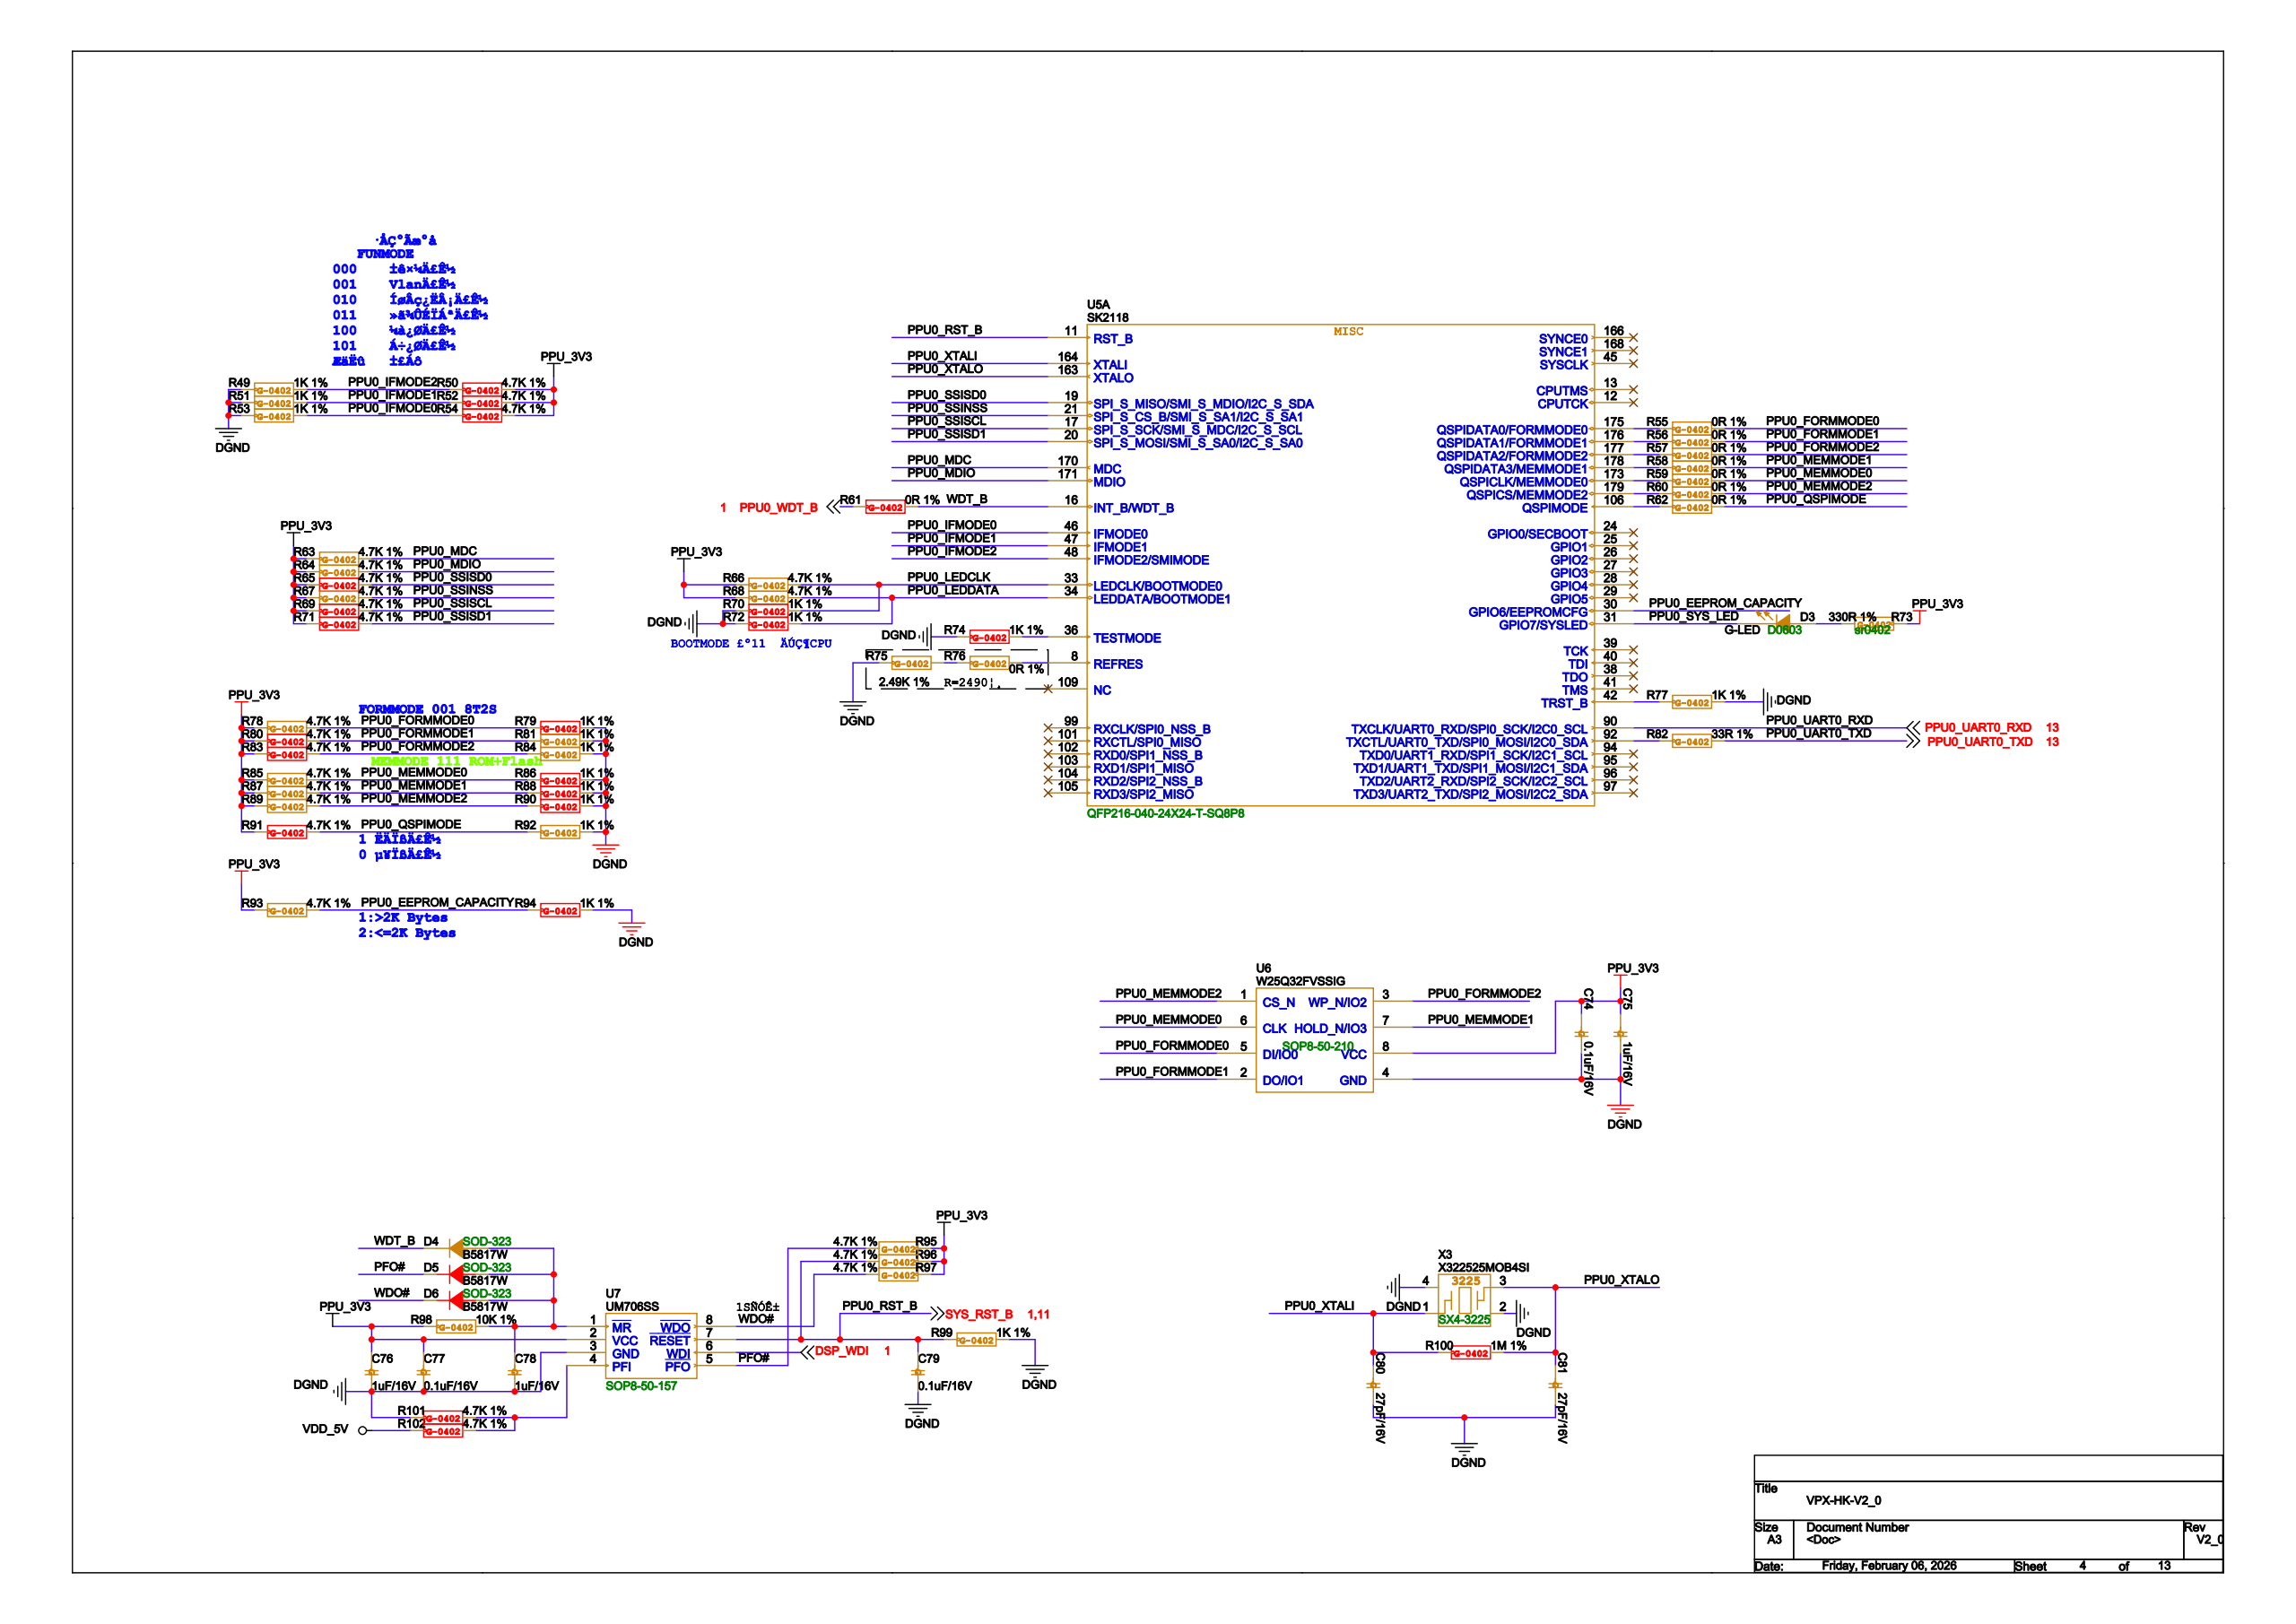Circuit board | Cadence Allegro | 598 parts | 541 nets | one sheet of the schematic
Parts on this sheet (reference | value | footprint):
C74 | 0.1uF/16V | SC0402
C75 | 1uF/16V | SC0402
C80 | 27pF/16V | SC0402
C81 | 27pF/16V | SC0402
D3 | G-LED | D0603
D4 | B5817W | SOD-323
D5 | B5817W | SOD-323
D6 | B5817W | SOD-323
R49 | 1K 1% | SR0402
R50 | 4.7K 1% | SR0402
R51 | 1K 1% | SR0402
R52 | 4.7K 1% | SR0402
R53 | 1K 1% | SR0402
R54 | 4.7K 1% | SR0402
R55 | 0R 1% | SR0402
R56 | 0R 1% | SR0402
R57 | 0R 1% | SR0402
R58 | 0R 1% | SR0402
R59 | 0R 1% | SR0402
R60 | 0R 1% | SR0402
R61 | 0R 1% | SR0402
R62 | 0R 1% | SR0402
R63 | 4.7K 1% | SR0402
R64 | 4.7K 1% | SR0402
R65 | 4.7K 1% | SR0402
R66 | 4.7K 1% | SR0402
R67 | 4.7K 1% | SR0402
R68 | 4.7K 1% | SR0402
R69 | 4.7K 1% | SR0402
R70 | 1K 1% | SR0402
R71 | 4.7K 1% | SR0402
R72 | 1K 1% | SR0402
R73 | 330R 1% | SR0402
R74 | 1K 1% | SR0402
R75 | 2.49K 1% | SR0402
R76 | 0R 1% | SR0402
R77 | 1K 1% | SR0402
R78 | 4.7K 1% | SR0402
R79 | 1K 1% | SR0402
R80 | 4.7K 1% | SR0402
R81 | 1K 1% | SR0402
R82 | 33R 1% | SR0402
R83 | 4.7K 1% | SR0402
R84 | 1K 1% | SR0402
R85 | 4.7K 1% | SR0402
R86 | 1K 1% | SR0402
R87 | 4.7K 1% | SR0402
R88 | 1K 1% | SR0402
R89 | 4.7K 1% | SR0402
R90 | 1K 1% | SR0402
R91 | 4.7K 1% | SR0402
R92 | 1K 1% | SR0402
R93 | 4.7K 1% | SR0402
R94 | 1K 1% | SR0402
R95 | 4.7K 1% | SR0402
R96 | 4.7K 1% | SR0402
R97 | 4.7K 1% | SR0402
R98 | 10K 1% | SR0402
R99 | 1K 1% | SR0402
R100 | 1M 1% | SR0402
R101 | 4.7K 1% | SR0402
R102 | 4.7K 1% | SR0402
U5 | SK2118 | QFP216-040-24X24-T-SQ8P8
U6 | W25Q32FVSSIG | SOP8-50-210
U7 | UM706SS | SOP8-50-157
X3 | X322525MOB4SI | SX4-3225
Nets of these parts (net: part-pin ...):
PPU_3V3: C74-1 C75-1 R50-2 R52-2 R54-2 R63-1 R64-1 R65-1 R66-1 R67-1 R68-1 R69-1 R71-1 R73-1 R78-1 R80-1 R83-1 R85-1 R87-1 R89-1 R91-1 R93-1 R95-1 R96-1 R97-1 R98-1 U6-8 U7-2
DGND: C74-2 C75-2 C80-2 C81-2 R49-1 R51-1 R53-1 R70-1 R72-1 R74-1 R75-1 R77-2 R79-2 R81-2 R84-2 R86-2 R88-2 R90-2 R92-2 R94-2 R99-2 R101-1 U6-4 U7-3 X3-2 X3-4 U5-7
VDD_5V: R102-1
N32613632: D4-2 D5-2 D6-2 R98-2 U7-1
PPU0_XTALI: C80-1 R100-1 X3-1 U5-164
PPU0_XTALO: C81-1 R100-2 X3-3 U5-163
DSP_WDI: U7-6
SYS_RST_B: R96-2 R99-1 U7-7 U5-11
WDT_B: D4-1 R61-2 U5-16
PFO#: D5-1 R95-2 U7-5
WDO#: D6-1 R97-2 U7-8
PPU0_UART0_TXD: R82-2
PPU0_UART0_RXD: U5-90
PPU0_WDT_B: R61-1
PPU0_EEPROM_CAPACITY: R93-2 R94-1 U5-30
PPU0_SYS_LED: D3-2 U5-31
PPU0_IFMODE0: R53-2 R54-1 U5-46
PPU0_IFMODE1: R51-2 R52-1 U5-47
PPU0_IFMODE2: R49-2 R50-1 U5-48
PPU0_LEDCLK: R66-2 R70-2 U5-33
PPU0_LEDDATA: R68-2 R72-2 U5-34
PPU0_MDC: R63-2 U5-170
PPU0_MDIO: R64-2 U5-171
N32613337: R59-1 U5-173
N32613339: R60-1 U5-179
N32613289: R55-1 U5-175
N32613291: R56-1 U5-176
N32613301: R57-1 U5-177
N32613319: R58-1 U5-178
N32613365: R62-1 U5-106
N32613186: R76-2 U5-8
PPU0_SSINSS: R67-2 U5-21
PPU0_SSISD0: R65-2 U5-19
PPU0_SSISD1: R71-2 U5-20
PPU0_SSISCL: R69-2 U5-17
N32613353: R74-2 U5-36
N32613188: R77-1 U5-42
N32613392: R82-1 U5-92
N32843620: R101-2 R102-2 U7-4
N32915429: D3-1 R73-2
PPU0_FORMMODE0: R55-2 R78-2 R79-1 U6-5
PPU0_FORMMODE1: R56-2 R80-2 R81-1 U6-2
PPU0_FORMMODE2: R57-2 R83-2 R84-1 U6-3
PPU0_MEMMODE0: R59-2 R85-2 R86-1 U6-6
PPU0_MEMMODE1: R58-2 R87-2 R88-1 U6-7
PPU0_MEMMODE2: R60-2 R89-2 R90-1 U6-1
PPU0_QSPIMODE: R62-2 R91-2 R92-1
N33441755: R75-2 R76-1